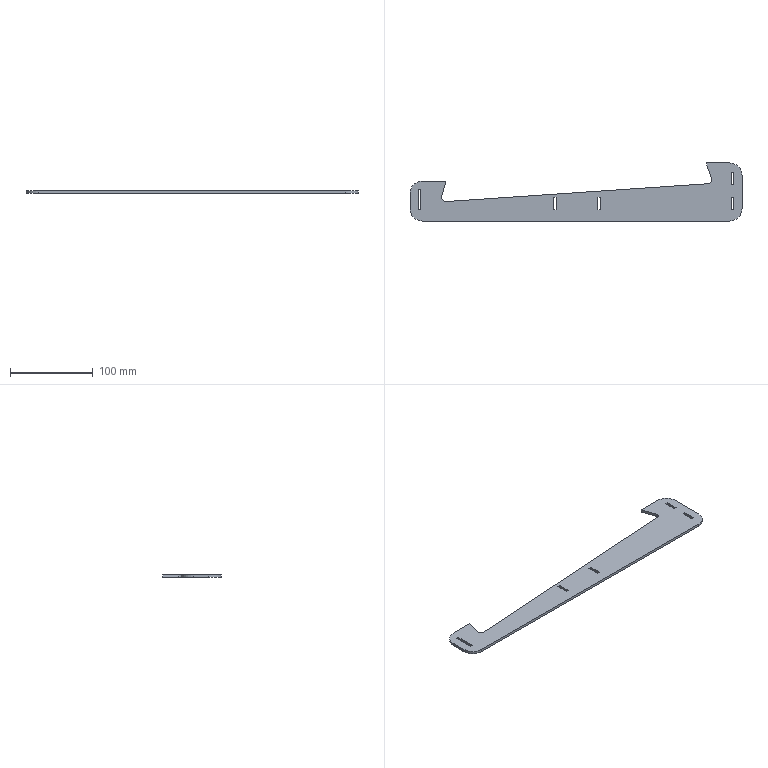Part | SolidWorks | features FlatPattern 1, SMBaseFlange 1, SheetMetal 1 | 1 solid | 36 faces | box 400 x 70 x 3.2 mm | volume 48547 mm3 | plane 29 | cylinder 4 | spline 3 | commonest cylinder face diameters 30 x4
STEP:
#1=CARTESIAN_POINT('',(187.397,-161.486,3.2));
#2=VERTEX_POINT('',#1);
#3=CARTESIAN_POINT('',(182.437,-167.928,3.2));
#4=VERTEX_POINT('',#3);
#5=CARTESIAN_POINT('',(187.397,-161.486,3.2));
#6=CARTESIAN_POINT('',(187.466,-161.697,3.2));
#7=CARTESIAN_POINT('',(187.548,-161.997,3.2));
#8=CARTESIAN_POINT('',(187.606,-162.322,3.2));
#9=CARTESIAN_POINT('',(187.625,-162.479,3.2));
#10=CARTESIAN_POINT('',(187.633,-162.555,3.2));
#11=CARTESIAN_POINT('',(187.635,-162.588,3.2));
#12=CARTESIAN_POINT('',(187.637,-162.609,3.2));
#13=CARTESIAN_POINT('',(187.638,-162.619,3.2));
#14=CARTESIAN_POINT('',(187.651,-162.822,3.2));
#15=CARTESIAN_POINT('',(187.65,-163.111,3.2));
#16=CARTESIAN_POINT('',(187.614,-163.449,3.2));
#17=CARTESIAN_POINT('',(187.591,-163.594,3.2));
#18=CARTESIAN_POINT('',(187.575,-163.691,3.2));
#19=CARTESIAN_POINT('',(187.565,-163.741,3.2));
#20=CARTESIAN_POINT('',(187.476,-164.167,3.2));
#21=CARTESIAN_POINT('',(187.29,-164.713,3.2));
#22=CARTESIAN_POINT('',(186.955,-165.309,3.2));
#23=CARTESIAN_POINT('',(186.758,-165.597,3.2));
#24=CARTESIAN_POINT('',(186.652,-165.738,3.2));
#25=CARTESIAN_POINT('',(186.605,-165.799,3.2));
#26=CARTESIAN_POINT('',(186.573,-165.838,3.2));
#27=CARTESIAN_POINT('',(186.557,-165.859,3.2));
#28=CARTESIAN_POINT('',(186.294,-166.181,3.2));
#29=CARTESIAN_POINT('',(185.879,-166.59,3.2));
#30=CARTESIAN_POINT('',(185.317,-166.988,3.2));
#31=CARTESIAN_POINT('',(185.06,-167.142,3.2));
#32=CARTESIAN_POINT('',(184.885,-167.24,3.2));
#33=CARTESIAN_POINT('',(184.794,-167.288,3.2));
#34=CARTESIAN_POINT('',(184.524,-167.423,3.2));
#35=CARTESIAN_POINT('',(184.251,-167.54,3.2));
#36=CARTESIAN_POINT('',(183.927,-167.648,3.2));
#37=CARTESIAN_POINT('',(183.764,-167.695,3.2));
#38=CARTESIAN_POINT('',(183.682,-167.717,3.2));
#39=CARTESIAN_POINT('',(183.641,-167.727,3.2));
#40=CARTESIAN_POINT('',(183.623,-167.731,3.2));
#41=CARTESIAN_POINT('',(183.611,-167.734,3.2));
#42=CARTESIAN_POINT('',(183.603,-167.736,3.2));
#43=CARTESIAN_POINT('',(183.346,-167.797,3.2));
#44=CARTESIAN_POINT('',(182.958,-167.861,3.2));
#45=CARTESIAN_POINT('',(182.437,-167.928,3.2));
#46=B_SPLINE_CURVE_WITH_KNOTS('',3,(#5,#6,#7,#8,#9,#10,#11,#12,#13,#14,#15,#16,#17,#18,#19,#20,#21,#22,#23,#24,#25,#26,#27,#28,#29,#30,#31,#32,#33,#34,#35,#36,#37,#38,#39,#40,#41,#42,#43,#44,#45),.UNSPECIFIED.,.F.,.F.,(4,1,1,1,1,2,2,1,1,2,2,1,1,1,1,2,2,1,1,2,2,1,1,1,1,1,2,2,4),(0.,0.0625,0.09375,0.1094,0.1172,0.1211,0.125,0.1875,0.2188,0.2344,0.25,0.375,0.4375,0.4688,0.4844,0.4922,0.5,0.625,0.6875,0.7188,0.75,0.8125,0.8438,0.8594,0.8672,0.8711,0.873,0.875,1.),.UNSPECIFIED.);
#47=EDGE_CURVE('',#2,#4,#46,.T.);
#48=ORIENTED_EDGE('',*,*,#47,.T.);
#49=CARTESIAN_POINT('',(-132.11,-189.357,3.2));
#50=VERTEX_POINT('',#49);
#51=CARTESIAN_POINT('',(182.437,-167.928,3.2));
#52=CARTESIAN_POINT('',(77.588,-175.071,3.2));
#53=CARTESIAN_POINT('',(-27.261,-182.214,3.2));
#54=CARTESIAN_POINT('',(-132.11,-189.357,3.2));
#55=B_SPLINE_CURVE_WITH_KNOTS('',3,(#51,#52,#53,#54),.UNSPECIFIED.,.F.,.F.,(4,4),(0.,1.),.UNSPECIFIED.);
#56=EDGE_CURVE('',#4,#50,#55,.T.);
#57=ORIENTED_EDGE('',*,*,#56,.T.);
#58=CARTESIAN_POINT('',(-137.953,-183.594,3.2));
#59=VERTEX_POINT('',#58);
#60=CARTESIAN_POINT('',(-132.11,-189.357,3.2));
#61=CARTESIAN_POINT('',(-132.532,-189.381,3.2));
#62=CARTESIAN_POINT('',(-133.143,-189.364,3.2));
#63=CARTESIAN_POINT('',(-133.815,-189.25,3.2));
#64=CARTESIAN_POINT('',(-134.141,-189.169,3.2));
#65=CARTESIAN_POINT('',(-134.302,-189.122,3.2));
#66=CARTESIAN_POINT('',(-134.37,-189.101,3.2));
#67=CARTESIAN_POINT('',(-134.416,-189.087,3.2));
#68=CARTESIAN_POINT('',(-134.437,-189.08,3.2));
#69=CARTESIAN_POINT('',(-134.848,-188.944,3.2));
#70=CARTESIAN_POINT('',(-135.394,-188.697,3.2));
#71=CARTESIAN_POINT('',(-135.969,-188.316,3.2));
#72=CARTESIAN_POINT('',(-136.242,-188.101,3.2));
#73=CARTESIAN_POINT('',(-136.355,-188.004,3.2));
#74=CARTESIAN_POINT('',(-136.43,-187.938,3.2));
#75=CARTESIAN_POINT('',(-136.466,-187.906,3.2));
#76=CARTESIAN_POINT('',(-136.809,-187.588,3.2));
#77=CARTESIAN_POINT('',(-137.202,-187.132,3.2));
#78=CARTESIAN_POINT('',(-137.545,-186.546,3.2));
#79=CARTESIAN_POINT('',(-137.688,-186.239,3.2));
#80=CARTESIAN_POINT('',(-137.743,-186.104,3.2));
#81=CARTESIAN_POINT('',(-137.778,-186.014,3.2));
#82=CARTESIAN_POINT('',(-137.795,-185.97,3.2));
#83=CARTESIAN_POINT('',(-137.879,-185.734,3.2));
#84=CARTESIAN_POINT('',(-137.932,-185.544,3.2));
#85=CARTESIAN_POINT('',(-138.012,-185.161,3.2));
#86=CARTESIAN_POINT('',(-138.038,-184.969,3.2));
#87=CARTESIAN_POINT('',(-138.057,-184.675,3.2));
#88=CARTESIAN_POINT('',(-138.061,-184.528,3.2));
#89=CARTESIAN_POINT('',(-138.057,-184.38,3.2));
#90=CARTESIAN_POINT('',(-138.052,-184.281,3.2));
#91=CARTESIAN_POINT('',(-138.05,-184.24,3.2));
#92=CARTESIAN_POINT('',(-138.031,-184.015,3.2));
#93=CARTESIAN_POINT('',(-138.,-183.815,3.2));
#94=CARTESIAN_POINT('',(-137.953,-183.594,3.2));
#95=B_SPLINE_CURVE_WITH_KNOTS('',3,(#60,#61,#62,#63,#64,#65,#66,#67,#68,#69,#70,#71,#72,#73,#74,#75,#76,#77,#78,#79,#80,#81,#82,#83,#84,#85,#86,#87,#88,#89,#90,#91,#92,#93,#94),.UNSPECIFIED.,.F.,.F.,(4,1,1,1,1,2,2,1,1,1,2,2,1,1,1,2,2,2,2,1,2,2,4),(0.,0.125,0.1875,0.2187,0.2344,0.2422,0.25,0.375,0.4375,0.4687,0.4844,0.5,0.625,0.6875,0.7187,0.7344,0.75,0.8125,0.875,0.9062,0.9219,0.9375,1.),.UNSPECIFIED.);
#96=EDGE_CURVE('',#50,#59,#95,.T.);
#97=ORIENTED_EDGE('',*,*,#96,.T.);
#98=CARTESIAN_POINT('',(-132.905,-164.74,3.2));
#99=VERTEX_POINT('',#98);
#100=CARTESIAN_POINT('',(-137.953,-183.594,3.2));
#101=CARTESIAN_POINT('',(-136.27,-177.309,3.2));
#102=CARTESIAN_POINT('',(-134.588,-171.025,3.2));
#103=CARTESIAN_POINT('',(-132.905,-164.74,3.2));
#104=B_SPLINE_CURVE_WITH_KNOTS('',3,(#100,#101,#102,#103),.UNSPECIFIED.,.F.,.F.,(4,4),(0.,1.),.UNSPECIFIED.);
#105=EDGE_CURVE('',#59,#99,#104,.T.);
#106=ORIENTED_EDGE('',*,*,#105,.T.);
#107=CARTESIAN_POINT('',(-161.142,-164.74,3.2));
#108=VERTEX_POINT('',#107);
#109=CARTESIAN_POINT('',(-132.905,-164.74,3.2));
#110=DIRECTION('',(-1.,0.,0.));
#111=VECTOR('',#110,1000.);
#112=LINE('',#109,#111);
#113=EDGE_CURVE('',#99,#108,#112,.T.);
#114=ORIENTED_EDGE('',*,*,#113,.T.);
#115=CARTESIAN_POINT('',(-176.142,-179.74,3.2));
#116=VERTEX_POINT('',#115);
#117=CARTESIAN_POINT('',(-161.142,-179.74,3.2));
#118=DIRECTION('',(0.,0.,1.));
#119=DIRECTION('',(1.,0.,0.));
#120=AXIS2_PLACEMENT_3D('',#117,#118,#119);
#121=CIRCLE('',#120,15.);
#122=EDGE_CURVE('',#108,#116,#121,.T.);
#123=ORIENTED_EDGE('',*,*,#122,.T.);
#124=CARTESIAN_POINT('',(-176.142,-197.865,3.2));
#125=VERTEX_POINT('',#124);
#126=CARTESIAN_POINT('',(-176.142,-179.74,3.2));
#127=DIRECTION('',(0.,-1.,0.));
#128=VECTOR('',#127,1000.);
#129=LINE('',#126,#128);
#130=EDGE_CURVE('',#116,#125,#129,.T.);
#131=ORIENTED_EDGE('',*,*,#130,.T.);
#132=CARTESIAN_POINT('',(-161.142,-212.865,3.2));
#133=VERTEX_POINT('',#132);
#134=CARTESIAN_POINT('',(-161.142,-197.865,3.2));
#135=DIRECTION('',(0.,0.,1.));
#136=DIRECTION('',(1.,0.,0.));
#137=AXIS2_PLACEMENT_3D('',#134,#135,#136);
#138=CIRCLE('',#137,15.);
#139=EDGE_CURVE('',#125,#133,#138,.T.);
#140=ORIENTED_EDGE('',*,*,#139,.T.);
#141=CARTESIAN_POINT('',(208.858,-212.865,3.2));
#142=VERTEX_POINT('',#141);
#143=CARTESIAN_POINT('',(-161.142,-212.865,3.2));
#144=DIRECTION('',(1.,0.,0.));
#145=VECTOR('',#144,1000.);
#146=LINE('',#143,#145);
#147=EDGE_CURVE('',#133,#142,#146,.T.);
#148=ORIENTED_EDGE('',*,*,#147,.T.);
#149=CARTESIAN_POINT('',(223.858,-197.865,3.2));
#150=VERTEX_POINT('',#149);
#151=CARTESIAN_POINT('',(208.858,-197.865,3.2));
#152=DIRECTION('',(0.,0.,1.));
#153=DIRECTION('',(1.,0.,0.));
#154=AXIS2_PLACEMENT_3D('',#151,#152,#153);
#155=CIRCLE('',#154,15.);
#156=EDGE_CURVE('',#142,#150,#155,.T.);
#157=ORIENTED_EDGE('',*,*,#156,.T.);
#158=CARTESIAN_POINT('',(223.858,-157.865,3.2));
#159=VERTEX_POINT('',#158);
#160=CARTESIAN_POINT('',(223.858,-197.865,3.2));
#161=DIRECTION('',(0.,1.,0.));
#162=VECTOR('',#161,1000.);
#163=LINE('',#160,#162);
#164=EDGE_CURVE('',#150,#159,#163,.T.);
#165=ORIENTED_EDGE('',*,*,#164,.T.);
#166=CARTESIAN_POINT('',(208.858,-142.865,3.2));
#167=VERTEX_POINT('',#166);
#168=CARTESIAN_POINT('',(208.858,-157.865,3.2));
#169=DIRECTION('',(0.,0.,1.));
#170=DIRECTION('',(1.,0.,0.));
#171=AXIS2_PLACEMENT_3D('',#168,#169,#170);
#172=CIRCLE('',#171,15.);
#173=EDGE_CURVE('',#159,#167,#172,.T.);
#174=ORIENTED_EDGE('',*,*,#173,.T.);
#175=CARTESIAN_POINT('',(180.62,-142.865,3.2));
#176=VERTEX_POINT('',#175);
#177=CARTESIAN_POINT('',(208.858,-142.865,3.2));
#178=DIRECTION('',(-1.,0.,0.));
#179=VECTOR('',#178,1000.);
#180=LINE('',#177,#179);
#181=EDGE_CURVE('',#167,#176,#180,.T.);
#182=ORIENTED_EDGE('',*,*,#181,.T.);
#183=CARTESIAN_POINT('',(180.62,-142.865,3.2));
#184=CARTESIAN_POINT('',(184.003,-152.159,3.2));
#185=CARTESIAN_POINT('',(187.397,-161.486,3.2));
#186=B_SPLINE_CURVE_WITH_KNOTS('',2,(#183,#184,#185),.UNSPECIFIED.,.F.,.F.,(3,3),(0.5261,0.5262),.UNSPECIFIED.);
#187=EDGE_CURVE('',#176,#2,#186,.T.);
#188=ORIENTED_EDGE('',*,*,#187,.T.);
#189=EDGE_LOOP('',(#48,#57,#97,#106,#114,#123,#131,#140,#148,#157,#165,#174,#182,#188));
#190=FACE_OUTER_BOUND('',#189,.T.);
#191=CARTESIAN_POINT('',(-166.142,-199.357,3.2));
#192=VERTEX_POINT('',#191);
#193=CARTESIAN_POINT('',(-162.942,-199.357,3.2));
#194=VERTEX_POINT('',#193);
#195=CARTESIAN_POINT('',(-166.142,-199.357,3.2));
#196=DIRECTION('',(1.,0.,0.));
#197=VECTOR('',#196,1000.);
#198=LINE('',#195,#197);
#199=EDGE_CURVE('',#192,#194,#198,.T.);
#200=ORIENTED_EDGE('',*,*,#199,.F.);
#201=CARTESIAN_POINT('',(-166.142,-174.357,3.2));
#202=VERTEX_POINT('',#201);
#203=CARTESIAN_POINT('',(-166.142,-174.357,3.2));
#204=DIRECTION('',(0.,-1.,0.));
#205=VECTOR('',#204,1000.);
#206=LINE('',#203,#205);
#207=EDGE_CURVE('',#202,#192,#206,.T.);
#208=ORIENTED_EDGE('',*,*,#207,.F.);
#209=CARTESIAN_POINT('',(-162.942,-174.357,3.2));
#210=VERTEX_POINT('',#209);
#211=CARTESIAN_POINT('',(-166.142,-174.357,3.2));
#212=DIRECTION('',(-1.,0.,0.));
#213=VECTOR('',#212,1000.);
#214=LINE('',#211,#213);
#215=EDGE_CURVE('',#210,#202,#214,.T.);
#216=ORIENTED_EDGE('',*,*,#215,.F.);
#217=CARTESIAN_POINT('',(-162.942,-174.357,3.2));
#218=DIRECTION('',(0.,1.,0.));
#219=VECTOR('',#218,1000.);
#220=LINE('',#217,#219);
#221=EDGE_CURVE('',#194,#210,#220,.T.);
#222=ORIENTED_EDGE('',*,*,#221,.F.);
#223=EDGE_LOOP('',(#200,#208,#216,#222));
#224=FACE_BOUND('',#223,.T.);
#225=CARTESIAN_POINT('',(-3.2,-199.357,3.2));
#226=VERTEX_POINT('',#225);
#227=CARTESIAN_POINT('',(0.,-199.357,3.2));
#228=VERTEX_POINT('',#227);
#229=CARTESIAN_POINT('',(-3.2,-199.357,3.2));
#230=DIRECTION('',(1.,0.,0.));
#231=VECTOR('',#230,1000.);
#232=LINE('',#229,#231);
#233=EDGE_CURVE('',#226,#228,#232,.T.);
#234=ORIENTED_EDGE('',*,*,#233,.F.);
#235=CARTESIAN_POINT('',(-3.2,-184.357,3.2));
#236=VERTEX_POINT('',#235);
#237=CARTESIAN_POINT('',(-3.2,-184.357,3.2));
#238=DIRECTION('',(0.,-1.,0.));
#239=VECTOR('',#238,1000.);
#240=LINE('',#237,#239);
#241=EDGE_CURVE('',#236,#226,#240,.T.);
#242=ORIENTED_EDGE('',*,*,#241,.F.);
#243=CARTESIAN_POINT('',(0.,-184.357,3.2));
#244=VERTEX_POINT('',#243);
#245=CARTESIAN_POINT('',(-3.2,-184.357,3.2));
#246=DIRECTION('',(-1.,0.,0.));
#247=VECTOR('',#246,1000.);
#248=LINE('',#245,#247);
#249=EDGE_CURVE('',#244,#236,#248,.T.);
#250=ORIENTED_EDGE('',*,*,#249,.F.);
#251=CARTESIAN_POINT('',(0.,-184.357,3.2));
#252=DIRECTION('',(0.,1.,0.));
#253=VECTOR('',#252,1000.);
#254=LINE('',#251,#253);
#255=EDGE_CURVE('',#228,#244,#254,.T.);
#256=ORIENTED_EDGE('',*,*,#255,.F.);
#257=EDGE_LOOP('',(#234,#242,#250,#256));
#258=FACE_BOUND('',#257,.T.);
#259=CARTESIAN_POINT('',(50.,-199.357,3.2));
#260=VERTEX_POINT('',#259);
#261=CARTESIAN_POINT('',(53.2,-199.357,3.2));
#262=VERTEX_POINT('',#261);
#263=CARTESIAN_POINT('',(50.,-199.357,3.2));
#264=DIRECTION('',(1.,0.,0.));
#265=VECTOR('',#264,1000.);
#266=LINE('',#263,#265);
#267=EDGE_CURVE('',#260,#262,#266,.T.);
#268=ORIENTED_EDGE('',*,*,#267,.F.);
#269=CARTESIAN_POINT('',(50.,-184.357,3.2));
#270=VERTEX_POINT('',#269);
#271=CARTESIAN_POINT('',(50.,-184.357,3.2));
#272=DIRECTION('',(0.,-1.,0.));
#273=VECTOR('',#272,1000.);
#274=LINE('',#271,#273);
#275=EDGE_CURVE('',#270,#260,#274,.T.);
#276=ORIENTED_EDGE('',*,*,#275,.F.);
#277=CARTESIAN_POINT('',(53.2,-184.357,3.2));
#278=VERTEX_POINT('',#277);
#279=CARTESIAN_POINT('',(50.,-184.357,3.2));
#280=DIRECTION('',(-1.,0.,0.));
#281=VECTOR('',#280,1000.);
#282=LINE('',#279,#281);
#283=EDGE_CURVE('',#278,#270,#282,.T.);
#284=ORIENTED_EDGE('',*,*,#283,.F.);
#285=CARTESIAN_POINT('',(53.2,-184.357,3.2));
#286=DIRECTION('',(0.,1.,0.));
#287=VECTOR('',#286,1000.);
#288=LINE('',#285,#287);
#289=EDGE_CURVE('',#262,#278,#288,.T.);
#290=ORIENTED_EDGE('',*,*,#289,.F.);
#291=EDGE_LOOP('',(#268,#276,#284,#290));
#292=FACE_BOUND('',#291,.T.);
#293=CARTESIAN_POINT('',(210.658,-169.357,3.2));
#294=VERTEX_POINT('',#293);
#295=CARTESIAN_POINT('',(213.858,-169.357,3.2));
#296=VERTEX_POINT('',#295);
#297=CARTESIAN_POINT('',(210.658,-169.357,3.2));
#298=DIRECTION('',(1.,0.,0.));
#299=VECTOR('',#298,1000.);
#300=LINE('',#297,#299);
#301=EDGE_CURVE('',#294,#296,#300,.T.);
#302=ORIENTED_EDGE('',*,*,#301,.F.);
#303=CARTESIAN_POINT('',(210.658,-154.357,3.2));
#304=VERTEX_POINT('',#303);
#305=CARTESIAN_POINT('',(210.658,-154.357,3.2));
#306=DIRECTION('',(0.,-1.,0.));
#307=VECTOR('',#306,1000.);
#308=LINE('',#305,#307);
#309=EDGE_CURVE('',#304,#294,#308,.T.);
#310=ORIENTED_EDGE('',*,*,#309,.F.);
#311=CARTESIAN_POINT('',(213.858,-154.357,3.2));
#312=VERTEX_POINT('',#311);
#313=CARTESIAN_POINT('',(210.658,-154.357,3.2));
#314=DIRECTION('',(-1.,0.,0.));
#315=VECTOR('',#314,1000.);
#316=LINE('',#313,#315);
#317=EDGE_CURVE('',#312,#304,#316,.T.);
#318=ORIENTED_EDGE('',*,*,#317,.F.);
#319=CARTESIAN_POINT('',(213.858,-154.357,3.2));
#320=DIRECTION('',(0.,1.,0.));
#321=VECTOR('',#320,1000.);
#322=LINE('',#319,#321);
#323=EDGE_CURVE('',#296,#312,#322,.T.);
#324=ORIENTED_EDGE('',*,*,#323,.F.);
#325=EDGE_LOOP('',(#302,#310,#318,#324));
#326=FACE_BOUND('',#325,.T.);
#327=CARTESIAN_POINT('',(210.658,-199.357,3.2));
#328=VERTEX_POINT('',#327);
#329=CARTESIAN_POINT('',(213.858,-199.357,3.2));
#330=VERTEX_POINT('',#329);
#331=CARTESIAN_POINT('',(210.658,-199.357,3.2));
#332=DIRECTION('',(1.,0.,0.));
#333=VECTOR('',#332,1000.);
#334=LINE('',#331,#333);
#335=EDGE_CURVE('',#328,#330,#334,.T.);
#336=ORIENTED_EDGE('',*,*,#335,.F.);
#337=CARTESIAN_POINT('',(210.658,-184.357,3.2));
#338=VERTEX_POINT('',#337);
#339=CARTESIAN_POINT('',(210.658,-184.357,3.2));
#340=DIRECTION('',(0.,-1.,0.));
#341=VECTOR('',#340,1000.);
#342=LINE('',#339,#341);
#343=EDGE_CURVE('',#338,#328,#342,.T.);
#344=ORIENTED_EDGE('',*,*,#343,.F.);
#345=CARTESIAN_POINT('',(213.858,-184.357,3.2));
#346=VERTEX_POINT('',#345);
#347=CARTESIAN_POINT('',(210.658,-184.357,3.2));
#348=DIRECTION('',(-1.,0.,0.));
#349=VECTOR('',#348,1000.);
#350=LINE('',#347,#349);
#351=EDGE_CURVE('',#346,#338,#350,.T.);
#352=ORIENTED_EDGE('',*,*,#351,.F.);
#353=CARTESIAN_POINT('',(213.858,-184.357,3.2));
#354=DIRECTION('',(0.,1.,0.));
#355=VECTOR('',#354,1000.);
#356=LINE('',#353,#355);
#357=EDGE_CURVE('',#330,#346,#356,.T.);
#358=ORIENTED_EDGE('',*,*,#357,.F.);
#359=EDGE_LOOP('',(#336,#344,#352,#358));
#360=FACE_BOUND('',#359,.T.);
#361=CARTESIAN_POINT('',(186.541,-165.878,3.2));
#362=DIRECTION('',(0.,0.,1.));
#363=DIRECTION('',(1.,0.,0.));
#364=AXIS2_PLACEMENT_3D('',#361,#362,#363);
#365=PLANE('',#364);
#366=ADVANCED_FACE('',(#190,#224,#258,#292,#326,#360),#365,.T.);
#367=CARTESIAN_POINT('',(210.658,-154.357,0.));
#368=VERTEX_POINT('',#367);
#369=CARTESIAN_POINT('',(210.658,-169.357,0.));
#370=VERTEX_POINT('',#369);
#371=CARTESIAN_POINT('',(210.658,-154.357,0.));
#372=DIRECTION('',(0.,-1.,0.));
#373=VECTOR('',#372,1000.);
#374=LINE('',#371,#373);
#375=EDGE_CURVE('',#368,#370,#374,.T.);
#376=ORIENTED_EDGE('',*,*,#375,.T.);
#377=CARTESIAN_POINT('',(213.858,-169.357,0.));
#378=VERTEX_POINT('',#377);
#379=CARTESIAN_POINT('',(210.658,-169.357,0.));
#380=DIRECTION('',(1.,0.,0.));
#381=VECTOR('',#380,1000.);
#382=LINE('',#379,#381);
#383=EDGE_CURVE('',#370,#378,#382,.T.);
#384=ORIENTED_EDGE('',*,*,#383,.T.);
#385=CARTESIAN_POINT('',(213.858,-154.357,0.));
#386=VERTEX_POINT('',#385);
#387=CARTESIAN_POINT('',(213.858,-154.357,0.));
#388=DIRECTION('',(0.,1.,0.));
#389=VECTOR('',#388,1000.);
#390=LINE('',#387,#389);
#391=EDGE_CURVE('',#378,#386,#390,.T.);
#392=ORIENTED_EDGE('',*,*,#391,.T.);
#393=CARTESIAN_POINT('',(210.658,-154.357,0.));
#394=DIRECTION('',(-1.,0.,0.));
#395=VECTOR('',#394,1000.);
#396=LINE('',#393,#395);
#397=EDGE_CURVE('',#386,#368,#396,.T.);
#398=ORIENTED_EDGE('',*,*,#397,.T.);
#399=EDGE_LOOP('',(#376,#384,#392,#398));
#400=FACE_BOUND('',#399,.T.);
#401=CARTESIAN_POINT('',(-3.2,-184.357,0.));
#402=VERTEX_POINT('',#401);
#403=CARTESIAN_POINT('',(-3.2,-199.357,0.));
#404=VERTEX_POINT('',#403);
#405=CARTESIAN_POINT('',(-3.2,-184.357,0.));
#406=DIRECTION('',(0.,-1.,0.));
#407=VECTOR('',#406,1000.);
#408=LINE('',#405,#407);
#409=EDGE_CURVE('',#402,#404,#408,.T.);
#410=ORIENTED_EDGE('',*,*,#409,.T.);
#411=CARTESIAN_POINT('',(0.,-199.357,0.));
#412=VERTEX_POINT('',#411);
#413=CARTESIAN_POINT('',(-3.2,-199.357,0.));
#414=DIRECTION('',(1.,0.,0.));
#415=VECTOR('',#414,1000.);
#416=LINE('',#413,#415);
#417=EDGE_CURVE('',#404,#412,#416,.T.);
#418=ORIENTED_EDGE('',*,*,#417,.T.);
#419=CARTESIAN_POINT('',(0.,-184.357,0.));
#420=VERTEX_POINT('',#419);
#421=CARTESIAN_POINT('',(0.,-184.357,0.));
#422=DIRECTION('',(0.,1.,0.));
#423=VECTOR('',#422,1000.);
#424=LINE('',#421,#423);
#425=EDGE_CURVE('',#412,#420,#424,.T.);
#426=ORIENTED_EDGE('',*,*,#425,.T.);
#427=CARTESIAN_POINT('',(-3.2,-184.357,0.));
#428=DIRECTION('',(-1.,0.,0.));
#429=VECTOR('',#428,1000.);
#430=LINE('',#427,#429);
#431=EDGE_CURVE('',#420,#402,#430,.T.);
#432=ORIENTED_EDGE('',*,*,#431,.T.);
#433=EDGE_LOOP('',(#410,#418,#426,#432));
#434=FACE_BOUND('',#433,.T.);
#435=CARTESIAN_POINT('',(187.397,-161.486,0.));
#436=VERTEX_POINT('',#435);
#437=CARTESIAN_POINT('',(182.437,-167.928,0.));
#438=VERTEX_POINT('',#437);
#439=CARTESIAN_POINT('',(187.397,-161.486,0.));
#440=CARTESIAN_POINT('',(187.445,-161.632,0.));
#441=CARTESIAN_POINT('',(187.544,-161.932,0.));
#442=CARTESIAN_POINT('',(187.628,-162.413,0.));
#443=CARTESIAN_POINT('',(187.659,-162.932,0.));
#444=CARTESIAN_POINT('',(187.61,-163.626,0.));
#445=CARTESIAN_POINT('',(187.39,-164.497,0.));
#446=CARTESIAN_POINT('',(186.881,-165.491,0.));
#447=CARTESIAN_POINT('',(186.11,-166.411,0.));
#448=CARTESIAN_POINT('',(185.064,-167.197,0.));
#449=CARTESIAN_POINT('',(183.813,-167.752,0.));
#450=CARTESIAN_POINT('',(182.885,-167.87,0.));
#451=CARTESIAN_POINT('',(182.437,-167.928,0.));
#452=B_SPLINE_CURVE_WITH_KNOTS('',3,(#439,#440,#441,#442,#443,#444,#445,#446,#447,#448,#449,#450,#451),.UNSPECIFIED.,.F.,.F.,(4,1,1,1,1,1,1,1,1,1,4),(0.,0.04871,0.1004,0.1558,0.2156,0.3245,0.4429,0.5702,0.7032,0.8565,1.),.UNSPECIFIED.);
#453=EDGE_CURVE('',#436,#438,#452,.T.);
#454=ORIENTED_EDGE('',*,*,#453,.F.);
#455=CARTESIAN_POINT('',(180.62,-142.865,0.));
#456=VERTEX_POINT('',#455);
#457=CARTESIAN_POINT('',(180.62,-142.865,0.));
#458=CARTESIAN_POINT('',(184.003,-152.159,0.));
#459=CARTESIAN_POINT('',(187.397,-161.486,0.));
#460=B_SPLINE_CURVE_WITH_KNOTS('',2,(#457,#458,#459),.UNSPECIFIED.,.F.,.F.,(3,3),(0.5261,0.5262),.UNSPECIFIED.);
#461=EDGE_CURVE('',#456,#436,#460,.T.);
#462=ORIENTED_EDGE('',*,*,#461,.F.);
#463=CARTESIAN_POINT('',(208.858,-142.865,0.));
#464=VERTEX_POINT('',#463);
#465=CARTESIAN_POINT('',(208.858,-142.865,0.));
#466=DIRECTION('',(-1.,0.,0.));
#467=VECTOR('',#466,1000.);
#468=LINE('',#465,#467);
#469=EDGE_CURVE('',#464,#456,#468,.T.);
#470=ORIENTED_EDGE('',*,*,#469,.F.);
#471=CARTESIAN_POINT('',(223.858,-157.865,0.));
#472=VERTEX_POINT('',#471);
#473=CARTESIAN_POINT('',(208.858,-157.865,0.));
#474=DIRECTION('',(0.,0.,1.));
#475=DIRECTION('',(1.,0.,0.));
#476=AXIS2_PLACEMENT_3D('',#473,#474,#475);
#477=CIRCLE('',#476,15.);
#478=EDGE_CURVE('',#472,#464,#477,.T.);
#479=ORIENTED_EDGE('',*,*,#478,.F.);
#480=CARTESIAN_POINT('',(223.858,-197.865,0.));
#481=VERTEX_POINT('',#480);
#482=CARTESIAN_POINT('',(223.858,-197.865,0.));
#483=DIRECTION('',(0.,1.,0.));
#484=VECTOR('',#483,1000.);
#485=LINE('',#482,#484);
#486=EDGE_CURVE('',#481,#472,#485,.T.);
#487=ORIENTED_EDGE('',*,*,#486,.F.);
#488=CARTESIAN_POINT('',(208.858,-212.865,0.));
#489=VERTEX_POINT('',#488);
#490=CARTESIAN_POINT('',(208.858,-197.865,0.));
#491=DIRECTION('',(0.,0.,1.));
#492=DIRECTION('',(1.,0.,0.));
#493=AXIS2_PLACEMENT_3D('',#490,#491,#492);
#494=CIRCLE('',#493,15.);
#495=EDGE_CURVE('',#489,#481,#494,.T.);
#496=ORIENTED_EDGE('',*,*,#495,.F.);
#497=CARTESIAN_POINT('',(-161.142,-212.865,0.));
#498=VERTEX_POINT('',#497);
#499=CARTESIAN_POINT('',(-161.142,-212.865,0.));
#500=DIRECTION('',(1.,0.,0.));
#501=VECTOR('',#500,1000.);
#502=LINE('',#499,#501);
#503=EDGE_CURVE('',#498,#489,#502,.T.);
#504=ORIENTED_EDGE('',*,*,#503,.F.);
#505=CARTESIAN_POINT('',(-176.142,-197.865,0.));
#506=VERTEX_POINT('',#505);
#507=CARTESIAN_POINT('',(-161.142,-197.865,0.));
#508=DIRECTION('',(0.,0.,1.));
#509=DIRECTION('',(1.,0.,0.));
#510=AXIS2_PLACEMENT_3D('',#507,#508,#509);
#511=CIRCLE('',#510,15.);
#512=EDGE_CURVE('',#506,#498,#511,.T.);
#513=ORIENTED_EDGE('',*,*,#512,.F.);
#514=CARTESIAN_POINT('',(-176.142,-179.74,0.));
#515=VERTEX_POINT('',#514);
#516=CARTESIAN_POINT('',(-176.142,-179.74,0.));
#517=DIRECTION('',(0.,-1.,0.));
#518=VECTOR('',#517,1000.);
#519=LINE('',#516,#518);
#520=EDGE_CURVE('',#515,#506,#519,.T.);
#521=ORIENTED_EDGE('',*,*,#520,.F.);
#522=CARTESIAN_POINT('',(-161.142,-164.74,0.));
#523=VERTEX_POINT('',#522);
#524=CARTESIAN_POINT('',(-161.142,-179.74,0.));
#525=DIRECTION('',(0.,0.,1.));
#526=DIRECTION('',(1.,0.,0.));
#527=AXIS2_PLACEMENT_3D('',#524,#525,#526);
#528=CIRCLE('',#527,15.);
#529=EDGE_CURVE('',#523,#515,#528,.T.);
#530=ORIENTED_EDGE('',*,*,#529,.F.);
#531=CARTESIAN_POINT('',(-132.905,-164.74,0.));
#532=VERTEX_POINT('',#531);
#533=CARTESIAN_POINT('',(-132.905,-164.74,0.));
#534=DIRECTION('',(-1.,0.,0.));
#535=VECTOR('',#534,1000.);
#536=LINE('',#533,#535);
#537=EDGE_CURVE('',#532,#523,#536,.T.);
#538=ORIENTED_EDGE('',*,*,#537,.F.);
#539=CARTESIAN_POINT('',(-137.953,-183.594,0.));
#540=VERTEX_POINT('',#539);
#541=CARTESIAN_POINT('',(-137.953,-183.594,0.));
#542=CARTESIAN_POINT('',(-136.27,-177.309,0.));
#543=CARTESIAN_POINT('',(-134.588,-171.025,0.));
#544=CARTESIAN_POINT('',(-132.905,-164.74,0.));
#545=B_SPLINE_CURVE_WITH_KNOTS('',3,(#541,#542,#543,#544),.UNSPECIFIED.,.F.,.F.,(4,4),(0.,1.),.UNSPECIFIED.);
#546=EDGE_CURVE('',#540,#532,#545,.T.);
#547=ORIENTED_EDGE('',*,*,#546,.F.);
#548=CARTESIAN_POINT('',(-132.11,-189.357,0.));
#549=VERTEX_POINT('',#548);
#550=CARTESIAN_POINT('',(-132.11,-189.357,0.));
#551=CARTESIAN_POINT('',(-132.186,-189.361,0.));
#552=CARTESIAN_POINT('',(-132.337,-189.37,0.));
#553=CARTESIAN_POINT('',(-132.567,-189.373,0.));
#554=CARTESIAN_POINT('',(-132.8,-189.369,0.));
#555=CARTESIAN_POINT('',(-133.037,-189.356,0.));
#556=CARTESIAN_POINT('',(-133.275,-189.333,0.));
#557=CARTESIAN_POINT('',(-133.654,-189.282,0.));
#558=CARTESIAN_POINT('',(-134.174,-189.172,0.));
#559=CARTESIAN_POINT('',(-135.008,-188.891,0.));
#560=CARTESIAN_POINT('',(-135.956,-188.375,0.));
#561=CARTESIAN_POINT('',(-136.744,-187.674,0.));
#562=CARTESIAN_POINT('',(-137.242,-187.044,0.));
#563=CARTESIAN_POINT('',(-137.548,-186.546,0.));
#564=CARTESIAN_POINT('',(-137.782,-186.036,0.));
#565=CARTESIAN_POINT('',(-137.947,-185.512,0.));
#566=CARTESIAN_POINT('',(-138.041,-184.996,0.));
#567=CARTESIAN_POINT('',(-138.066,-184.548,0.));
#568=CARTESIAN_POINT('',(-138.049,-184.178,0.));
#569=CARTESIAN_POINT('',(-138.013,-183.88,0.));
#570=CARTESIAN_POINT('',(-137.973,-183.688,0.));
#571=CARTESIAN_POINT('',(-137.953,-183.594,0.));
#572=B_SPLINE_CURVE_WITH_KNOTS('',3,(#550,#551,#552,#553,#554,#555,#556,#557,#558,#559,#560,#561,#562,#563,#564,#565,#566,#567,#568,#569,#570,#571),.UNSPECIFIED.,.F.,.F.,(4,1,1,1,1,1,1,1,1,1,1,1,1,1,1,1,1,1,1,4),(0.,0.02376,0.04786,0.07231,0.09712,0.1223,0.1479,0.2174,0.2893,0.4245,0.5536,0.618,0.6781,0.7387,0.7962,0.8526,0.9055,0.9385,0.9699,1.),.UNSPECIFIED.);
#573=EDGE_CURVE('',#549,#540,#572,.T.);
#574=ORIENTED_EDGE('',*,*,#573,.F.);
#575=CARTESIAN_POINT('',(182.437,-167.928,0.));
#576=CARTESIAN_POINT('',(77.588,-175.071,0.));
#577=CARTESIAN_POINT('',(-27.261,-182.214,0.));
#578=CARTESIAN_POINT('',(-132.11,-189.357,0.));
#579=B_SPLINE_CURVE_WITH_KNOTS('',3,(#575,#576,#577,#578),.UNSPECIFIED.,.F.,.F.,(4,4),(0.,1.),.UNSPECIFIED.);
#580=EDGE_CURVE('',#438,#549,#579,.T.);
#581=ORIENTED_EDGE('',*,*,#580,.F.);
#582=EDGE_LOOP('',(#454,#462,#470,#479,#487,#496,#504,#513,#521,#530,#538,#547,#574,#581));
#583=FACE_OUTER_BOUND('',#582,.T.);
#584=CARTESIAN_POINT('',(-166.142,-174.357,0.));
#585=VERTEX_POINT('',#584);
#586=CARTESIAN_POINT('',(-166.142,-199.357,0.));
#587=VERTEX_POINT('',#586);
#588=CARTESIAN_POINT('',(-166.142,-174.357,0.));
#589=DIRECTION('',(0.,-1.,0.));
#590=VECTOR('',#589,1000.);
#591=LINE('',#588,#590);
#592=EDGE_CURVE('',#585,#587,#591,.T.);
#593=ORIENTED_EDGE('',*,*,#592,.T.);
#594=CARTESIAN_POINT('',(-162.942,-199.357,0.));
#595=VERTEX_POINT('',#594);
#596=CARTESIAN_POINT('',(-166.142,-199.357,0.));
#597=DIRECTION('',(1.,0.,0.));
#598=VECTOR('',#597,1000.);
#599=LINE('',#596,#598);
#600=EDGE_CURVE('',#587,#595,#599,.T.);
#601=ORIENTED_EDGE('',*,*,#600,.T.);
#602=CARTESIAN_POINT('',(-162.942,-174.357,0.));
#603=VERTEX_POINT('',#602);
#604=CARTESIAN_POINT('',(-162.942,-174.357,0.));
#605=DIRECTION('',(0.,1.,0.));
#606=VECTOR('',#605,1000.);
#607=LINE('',#604,#606);
#608=EDGE_CURVE('',#595,#603,#607,.T.);
#609=ORIENTED_EDGE('',*,*,#608,.T.);
#610=CARTESIAN_POINT('',(-166.142,-174.357,0.));
#611=DIRECTION('',(-1.,0.,0.));
#612=VECTOR('',#611,1000.);
#613=LINE('',#610,#612);
#614=EDGE_CURVE('',#603,#585,#613,.T.);
#615=ORIENTED_EDGE('',*,*,#614,.T.);
#616=EDGE_LOOP('',(#593,#601,#609,#615));
#617=FACE_BOUND('',#616,.T.);
#618=CARTESIAN_POINT('',(50.,-184.357,0.));
#619=VERTEX_POINT('',#618);
#620=CARTESIAN_POINT('',(50.,-199.357,0.));
#621=VERTEX_POINT('',#620);
#622=CARTESIAN_POINT('',(50.,-184.357,0.));
#623=DIRECTION('',(0.,-1.,0.));
#624=VECTOR('',#623,1000.);
#625=LINE('',#622,#624);
#626=EDGE_CURVE('',#619,#621,#625,.T.);
#627=ORIENTED_EDGE('',*,*,#626,.T.);
#628=CARTESIAN_POINT('',(53.2,-199.357,0.));
#629=VERTEX_POINT('',#628);
#630=CARTESIAN_POINT('',(50.,-199.357,0.));
#631=DIRECTION('',(1.,0.,0.));
#632=VECTOR('',#631,1000.);
#633=LINE('',#630,#632);
#634=EDGE_CURVE('',#621,#629,#633,.T.);
#635=ORIENTED_EDGE('',*,*,#634,.T.);
#636=CARTESIAN_POINT('',(53.2,-184.357,0.));
#637=VERTEX_POINT('',#636);
#638=CARTESIAN_POINT('',(53.2,-184.357,0.));
#639=DIRECTION('',(0.,1.,0.));
#640=VECTOR('',#639,1000.);
#641=LINE('',#638,#640);
#642=EDGE_CURVE('',#629,#637,#641,.T.);
#643=ORIENTED_EDGE('',*,*,#642,.T.);
#644=CARTESIAN_POINT('',(50.,-184.357,0.));
#645=DIRECTION('',(-1.,0.,0.));
#646=VECTOR('',#645,1000.);
#647=LINE('',#644,#646);
#648=EDGE_CURVE('',#637,#619,#647,.T.);
#649=ORIENTED_EDGE('',*,*,#648,.T.);
#650=EDGE_LOOP('',(#627,#635,#643,#649));
#651=FACE_BOUND('',#650,.T.);
#652=CARTESIAN_POINT('',(210.658,-184.357,0.));
#653=VERTEX_POINT('',#652);
#654=CARTESIAN_POINT('',(210.658,-199.357,0.));
#655=VERTEX_POINT('',#654);
#656=CARTESIAN_POINT('',(210.658,-184.357,0.));
#657=DIRECTION('',(0.,-1.,0.));
#658=VECTOR('',#657,1000.);
#659=LINE('',#656,#658);
#660=EDGE_CURVE('',#653,#655,#659,.T.);
#661=ORIENTED_EDGE('',*,*,#660,.T.);
#662=CARTESIAN_POINT('',(213.858,-199.357,0.));
#663=VERTEX_POINT('',#662);
#664=CARTESIAN_POINT('',(210.658,-199.357,0.));
#665=DIRECTION('',(1.,0.,0.));
#666=VECTOR('',#665,1000.);
#667=LINE('',#664,#666);
#668=EDGE_CURVE('',#655,#663,#667,.T.);
#669=ORIENTED_EDGE('',*,*,#668,.T.);
#670=CARTESIAN_POINT('',(213.858,-184.357,0.));
#671=VERTEX_POINT('',#670);
#672=CARTESIAN_POINT('',(213.858,-184.357,0.));
#673=DIRECTION('',(0.,1.,0.));
#674=VECTOR('',#673,1000.);
#675=LINE('',#672,#674);
#676=EDGE_CURVE('',#663,#671,#675,.T.);
#677=ORIENTED_EDGE('',*,*,#676,.T.);
#678=CARTESIAN_POINT('',(210.658,-184.357,0.));
#679=DIRECTION('',(-1.,0.,0.));
#680=VECTOR('',#679,1000.);
#681=LINE('',#678,#680);
#682=EDGE_CURVE('',#671,#653,#681,.T.);
#683=ORIENTED_EDGE('',*,*,#682,.T.);
#684=EDGE_LOOP('',(#661,#669,#677,#683));
#685=FACE_BOUND('',#684,.T.);
#686=CARTESIAN_POINT('',(186.541,-165.878,0.));
#687=DIRECTION('',(0.,0.,1.));
#688=DIRECTION('',(1.,0.,0.));
#689=AXIS2_PLACEMENT_3D('',#686,#687,#688);
#690=PLANE('',#689);
#691=ADVANCED_FACE('',(#400,#434,#583,#617,#651,#685),#690,.F.);
#692=ORIENTED_EDGE('',*,*,#453,.T.);
#693=CARTESIAN_POINT('',(182.437,-167.928,3.2));
#694=DIRECTION('',(0.,0.,-1.));
#695=VECTOR('',#694,1000.);
#696=LINE('',#693,#695);
#697=EDGE_CURVE('',#4,#438,#696,.T.);
#698=ORIENTED_EDGE('',*,*,#697,.F.);
#699=ORIENTED_EDGE('',*,*,#47,.F.);
#700=CARTESIAN_POINT('',(187.397,-161.486,3.2));
#701=DIRECTION('',(0.,0.,-1.));
#702=VECTOR('',#701,1000.);
#703=LINE('',#700,#702);
#704=EDGE_CURVE('',#2,#436,#703,.T.);
#705=ORIENTED_EDGE('',*,*,#704,.T.);
#706=EDGE_LOOP('',(#692,#698,#699,#705));
#707=FACE_OUTER_BOUND('',#706,.T.);
#708=CARTESIAN_POINT('',(187.397,-161.486,3.2));
#709=CARTESIAN_POINT('',(187.397,-161.486,0.));
#710=CARTESIAN_POINT('',(187.445,-161.632,3.2));
#711=CARTESIAN_POINT('',(187.445,-161.632,0.));
#712=CARTESIAN_POINT('',(187.544,-161.932,3.2));
#713=CARTESIAN_POINT('',(187.544,-161.932,0.));
#714=CARTESIAN_POINT('',(187.628,-162.413,3.2));
#715=CARTESIAN_POINT('',(187.628,-162.413,0.));
#716=CARTESIAN_POINT('',(187.659,-162.932,3.2));
#717=CARTESIAN_POINT('',(187.659,-162.932,0.));
#718=CARTESIAN_POINT('',(187.61,-163.626,3.2));
#719=CARTESIAN_POINT('',(187.61,-163.626,0.));
#720=CARTESIAN_POINT('',(187.39,-164.497,3.2));
#721=CARTESIAN_POINT('',(187.39,-164.497,0.));
#722=CARTESIAN_POINT('',(186.881,-165.491,3.2));
#723=CARTESIAN_POINT('',(186.881,-165.491,0.));
#724=CARTESIAN_POINT('',(186.11,-166.411,3.2));
#725=CARTESIAN_POINT('',(186.11,-166.411,0.));
#726=CARTESIAN_POINT('',(185.064,-167.197,3.2));
#727=CARTESIAN_POINT('',(185.064,-167.197,0.));
#728=CARTESIAN_POINT('',(183.813,-167.752,3.2));
#729=CARTESIAN_POINT('',(183.813,-167.752,0.));
#730=CARTESIAN_POINT('',(182.885,-167.87,3.2));
#731=CARTESIAN_POINT('',(182.885,-167.87,0.));
#732=CARTESIAN_POINT('',(182.437,-167.928,3.2));
#733=CARTESIAN_POINT('',(182.437,-167.928,0.));
#734=B_SPLINE_SURFACE_WITH_KNOTS('',3,1,((#708,#709),(#710,#711),(#712,#713),(#714,#715),(#716,#717),(#718,#719),(#720,#721),(#722,#723),(#724,#725),(#726,#727),(#728,#729),(#730,#731),(#732,#733)),.UNSPECIFIED.,.F.,.F.,.F.,(4,1,1,1,1,1,1,1,1,1,4),(2,2),(0.,0.04871,0.1004,0.1558,0.2156,0.3245,0.4429,0.5702,0.7032,0.8565,1.),(0.,1.),.UNSPECIFIED.);
#735=ADVANCED_FACE('',(#707),#734,.F.);
#736=ORIENTED_EDGE('',*,*,#580,.T.);
#737=CARTESIAN_POINT('',(-132.11,-189.357,3.2));
#738=DIRECTION('',(0.,0.,-1.));
#739=VECTOR('',#738,1000.);
#740=LINE('',#737,#739);
#741=EDGE_CURVE('',#50,#549,#740,.T.);
#742=ORIENTED_EDGE('',*,*,#741,.F.);
#743=ORIENTED_EDGE('',*,*,#56,.F.);
#744=ORIENTED_EDGE('',*,*,#697,.T.);
#745=EDGE_LOOP('',(#736,#742,#743,#744));
#746=FACE_OUTER_BOUND('',#745,.T.);
#747=CARTESIAN_POINT('',(182.437,-167.928,3.2));
#748=DIRECTION('',(0.06797,-0.9977,0.));
#749=DIRECTION('',(0.9977,0.06797,0.));
#750=AXIS2_PLACEMENT_3D('',#747,#748,#749);
#751=PLANE('',#750);
#752=ADVANCED_FACE('',(#746),#751,.F.);
#753=ORIENTED_EDGE('',*,*,#573,.T.);
#754=CARTESIAN_POINT('',(-137.953,-183.594,3.2));
#755=DIRECTION('',(0.,0.,-1.));
#756=VECTOR('',#755,1000.);
#757=LINE('',#754,#756);
#758=EDGE_CURVE('',#59,#540,#757,.T.);
#759=ORIENTED_EDGE('',*,*,#758,.F.);
#760=ORIENTED_EDGE('',*,*,#96,.F.);
#761=ORIENTED_EDGE('',*,*,#741,.T.);
#762=EDGE_LOOP('',(#753,#759,#760,#761));
#763=FACE_OUTER_BOUND('',#762,.T.);
#764=CARTESIAN_POINT('',(-132.11,-189.357,3.2));
#765=CARTESIAN_POINT('',(-132.11,-189.357,0.));
#766=CARTESIAN_POINT('',(-132.186,-189.361,3.2));
#767=CARTESIAN_POINT('',(-132.186,-189.361,0.));
#768=CARTESIAN_POINT('',(-132.337,-189.37,3.2));
#769=CARTESIAN_POINT('',(-132.337,-189.37,0.));
#770=CARTESIAN_POINT('',(-132.567,-189.373,3.2));
#771=CARTESIAN_POINT('',(-132.567,-189.373,0.));
#772=CARTESIAN_POINT('',(-132.8,-189.369,3.2));
#773=CARTESIAN_POINT('',(-132.8,-189.369,0.));
#774=CARTESIAN_POINT('',(-133.037,-189.356,3.2));
#775=CARTESIAN_POINT('',(-133.037,-189.356,0.));
#776=CARTESIAN_POINT('',(-133.275,-189.333,3.2));
#777=CARTESIAN_POINT('',(-133.275,-189.333,0.));
#778=CARTESIAN_POINT('',(-133.654,-189.282,3.2));
#779=CARTESIAN_POINT('',(-133.654,-189.282,0.));
#780=CARTESIAN_POINT('',(-134.174,-189.172,3.2));
#781=CARTESIAN_POINT('',(-134.174,-189.172,0.));
#782=CARTESIAN_POINT('',(-135.008,-188.891,3.2));
#783=CARTESIAN_POINT('',(-135.008,-188.891,0.));
#784=CARTESIAN_POINT('',(-135.956,-188.375,3.2));
#785=CARTESIAN_POINT('',(-135.956,-188.375,0.));
#786=CARTESIAN_POINT('',(-136.744,-187.674,3.2));
#787=CARTESIAN_POINT('',(-136.744,-187.674,0.));
#788=CARTESIAN_POINT('',(-137.242,-187.044,3.2));
#789=CARTESIAN_POINT('',(-137.242,-187.044,0.));
#790=CARTESIAN_POINT('',(-137.548,-186.546,3.2));
#791=CARTESIAN_POINT('',(-137.548,-186.546,0.));
#792=CARTESIAN_POINT('',(-137.782,-186.036,3.2));
#793=CARTESIAN_POINT('',(-137.782,-186.036,0.));
#794=CARTESIAN_POINT('',(-137.947,-185.512,3.2));
#795=CARTESIAN_POINT('',(-137.947,-185.512,0.));
#796=CARTESIAN_POINT('',(-138.041,-184.996,3.2));
#797=CARTESIAN_POINT('',(-138.041,-184.996,0.));
#798=CARTESIAN_POINT('',(-138.066,-184.548,3.2));
#799=CARTESIAN_POINT('',(-138.066,-184.548,0.));
#800=CARTESIAN_POINT('',(-138.049,-184.178,3.2));
#801=CARTESIAN_POINT('',(-138.049,-184.178,0.));
#802=CARTESIAN_POINT('',(-138.013,-183.88,3.2));
#803=CARTESIAN_POINT('',(-138.013,-183.88,0.));
#804=CARTESIAN_POINT('',(-137.973,-183.688,3.2));
#805=CARTESIAN_POINT('',(-137.973,-183.688,0.));
#806=CARTESIAN_POINT('',(-137.953,-183.594,3.2));
#807=CARTESIAN_POINT('',(-137.953,-183.594,0.));
#808=B_SPLINE_SURFACE_WITH_KNOTS('',3,1,((#764,#765),(#766,#767),(#768,#769),(#770,#771),(#772,#773),(#774,#775),(#776,#777),(#778,#779),(#780,#781),(#782,#783),(#784,#785),(#786,#787),(#788,#789),(#790,#791),(#792,#793),(#794,#795),(#796,#797),(#798,#799),(#800,#801),(#802,#803),(#804,#805),(#806,#807)),.UNSPECIFIED.,.F.,.F.,.F.,(4,1,1,1,1,1,1,1,1,1,1,1,1,1,1,1,1,1,1,4),(2,2),(0.,0.02376,0.04786,0.07231,0.09712,0.1223,0.1479,0.2174,0.2893,0.4245,0.5536,0.618,0.6781,0.7387,0.7962,0.8526,0.9055,0.9385,0.9699,1.),(0.,1.),.UNSPECIFIED.);
#809=ADVANCED_FACE('',(#763),#808,.F.);
#810=ORIENTED_EDGE('',*,*,#546,.T.);
#811=CARTESIAN_POINT('',(-132.905,-164.74,3.2));
#812=DIRECTION('',(0.,0.,-1.));
#813=VECTOR('',#812,1000.);
#814=LINE('',#811,#813);
#815=EDGE_CURVE('',#99,#532,#814,.T.);
#816=ORIENTED_EDGE('',*,*,#815,.F.);
#817=ORIENTED_EDGE('',*,*,#105,.F.);
#818=ORIENTED_EDGE('',*,*,#758,.T.);
#819=EDGE_LOOP('',(#810,#816,#817,#818));
#820=FACE_OUTER_BOUND('',#819,.T.);
#821=CARTESIAN_POINT('',(-137.953,-183.594,3.2));
#822=DIRECTION('',(-0.966,0.2586,0.));
#823=DIRECTION('',(-0.2586,-0.966,0.));
#824=AXIS2_PLACEMENT_3D('',#821,#822,#823);
#825=PLANE('',#824);
#826=ADVANCED_FACE('',(#820),#825,.F.);
#827=ORIENTED_EDGE('',*,*,#537,.T.);
#828=CARTESIAN_POINT('',(-161.142,-164.74,3.2));
#829=DIRECTION('',(0.,0.,-1.));
#830=VECTOR('',#829,1000.);
#831=LINE('',#828,#830);
#832=EDGE_CURVE('',#108,#523,#831,.T.);
#833=ORIENTED_EDGE('',*,*,#832,.F.);
#834=ORIENTED_EDGE('',*,*,#113,.F.);
#835=ORIENTED_EDGE('',*,*,#815,.T.);
#836=EDGE_LOOP('',(#827,#833,#834,#835));
#837=FACE_OUTER_BOUND('',#836,.T.);
#838=CARTESIAN_POINT('',(-132.905,-164.74,3.2));
#839=DIRECTION('',(0.,-1.,0.));
#840=DIRECTION('',(1.,0.,0.));
#841=AXIS2_PLACEMENT_3D('',#838,#839,#840);
#842=PLANE('',#841);
#843=ADVANCED_FACE('',(#837),#842,.F.);
#844=ORIENTED_EDGE('',*,*,#529,.T.);
#845=CARTESIAN_POINT('',(-176.142,-179.74,3.2));
#846=DIRECTION('',(0.,0.,-1.));
#847=VECTOR('',#846,1000.);
#848=LINE('',#845,#847);
#849=EDGE_CURVE('',#116,#515,#848,.T.);
#850=ORIENTED_EDGE('',*,*,#849,.F.);
#851=ORIENTED_EDGE('',*,*,#122,.F.);
#852=ORIENTED_EDGE('',*,*,#832,.T.);
#853=EDGE_LOOP('',(#844,#850,#851,#852));
#854=FACE_OUTER_BOUND('',#853,.T.);
#855=CARTESIAN_POINT('',(-161.142,-179.74,3.2));
#856=DIRECTION('',(0.,0.,-1.));
#857=DIRECTION('',(-1.,0.,0.));
#858=AXIS2_PLACEMENT_3D('',#855,#856,#857);
#859=CYLINDRICAL_SURFACE('',#858,15.);
#860=ADVANCED_FACE('',(#854),#859,.T.);
#861=ORIENTED_EDGE('',*,*,#520,.T.);
#862=CARTESIAN_POINT('',(-176.142,-197.865,3.2));
#863=DIRECTION('',(0.,0.,-1.));
#864=VECTOR('',#863,1000.);
#865=LINE('',#862,#864);
#866=EDGE_CURVE('',#125,#506,#865,.T.);
#867=ORIENTED_EDGE('',*,*,#866,.F.);
#868=ORIENTED_EDGE('',*,*,#130,.F.);
#869=ORIENTED_EDGE('',*,*,#849,.T.);
#870=EDGE_LOOP('',(#861,#867,#868,#869));
#871=FACE_OUTER_BOUND('',#870,.T.);
#872=CARTESIAN_POINT('',(-176.142,-179.74,3.2));
#873=DIRECTION('',(1.,0.,0.));
#874=DIRECTION('',(0.,0.,-1.));
#875=AXIS2_PLACEMENT_3D('',#872,#873,#874);
#876=PLANE('',#875);
#877=ADVANCED_FACE('',(#871),#876,.F.);
#878=ORIENTED_EDGE('',*,*,#512,.T.);
#879=CARTESIAN_POINT('',(-161.142,-212.865,3.2));
#880=DIRECTION('',(0.,0.,-1.));
#881=VECTOR('',#880,1000.);
#882=LINE('',#879,#881);
#883=EDGE_CURVE('',#133,#498,#882,.T.);
#884=ORIENTED_EDGE('',*,*,#883,.F.);
#885=ORIENTED_EDGE('',*,*,#139,.F.);
#886=ORIENTED_EDGE('',*,*,#866,.T.);
#887=EDGE_LOOP('',(#878,#884,#885,#886));
#888=FACE_OUTER_BOUND('',#887,.T.);
#889=CARTESIAN_POINT('',(-161.142,-197.865,3.2));
#890=DIRECTION('',(0.,0.,-1.));
#891=DIRECTION('',(-1.,0.,0.));
#892=AXIS2_PLACEMENT_3D('',#889,#890,#891);
#893=CYLINDRICAL_SURFACE('',#892,15.);
#894=ADVANCED_FACE('',(#888),#893,.T.);
#895=ORIENTED_EDGE('',*,*,#503,.T.);
#896=CARTESIAN_POINT('',(208.858,-212.865,3.2));
#897=DIRECTION('',(0.,0.,-1.));
#898=VECTOR('',#897,1000.);
#899=LINE('',#896,#898);
#900=EDGE_CURVE('',#142,#489,#899,.T.);
#901=ORIENTED_EDGE('',*,*,#900,.F.);
#902=ORIENTED_EDGE('',*,*,#147,.F.);
#903=ORIENTED_EDGE('',*,*,#883,.T.);
#904=EDGE_LOOP('',(#895,#901,#902,#903));
#905=FACE_OUTER_BOUND('',#904,.T.);
#906=CARTESIAN_POINT('',(-161.142,-212.865,3.2));
#907=DIRECTION('',(0.,1.,0.));
#908=DIRECTION('',(0.,0.,1.));
#909=AXIS2_PLACEMENT_3D('',#906,#907,#908);
#910=PLANE('',#909);
#911=ADVANCED_FACE('',(#905),#910,.F.);
#912=ORIENTED_EDGE('',*,*,#495,.T.);
#913=CARTESIAN_POINT('',(223.858,-197.865,3.2));
#914=DIRECTION('',(0.,0.,-1.));
#915=VECTOR('',#914,1000.);
#916=LINE('',#913,#915);
#917=EDGE_CURVE('',#150,#481,#916,.T.);
#918=ORIENTED_EDGE('',*,*,#917,.F.);
#919=ORIENTED_EDGE('',*,*,#156,.F.);
#920=ORIENTED_EDGE('',*,*,#900,.T.);
#921=EDGE_LOOP('',(#912,#918,#919,#920));
#922=FACE_OUTER_BOUND('',#921,.T.);
#923=CARTESIAN_POINT('',(208.858,-197.865,3.2));
#924=DIRECTION('',(0.,0.,-1.));
#925=DIRECTION('',(-1.,0.,0.));
#926=AXIS2_PLACEMENT_3D('',#923,#924,#925);
#927=CYLINDRICAL_SURFACE('',#926,15.);
#928=ADVANCED_FACE('',(#922),#927,.T.);
#929=ORIENTED_EDGE('',*,*,#486,.T.);
#930=CARTESIAN_POINT('',(223.858,-157.865,3.2));
#931=DIRECTION('',(0.,0.,-1.));
#932=VECTOR('',#931,1000.);
#933=LINE('',#930,#932);
#934=EDGE_CURVE('',#159,#472,#933,.T.);
#935=ORIENTED_EDGE('',*,*,#934,.F.);
#936=ORIENTED_EDGE('',*,*,#164,.F.);
#937=ORIENTED_EDGE('',*,*,#917,.T.);
#938=EDGE_LOOP('',(#929,#935,#936,#937));
#939=FACE_OUTER_BOUND('',#938,.T.);
#940=CARTESIAN_POINT('',(223.858,-197.865,3.2));
#941=DIRECTION('',(-1.,0.,0.));
#942=DIRECTION('',(0.,-1.,0.));
#943=AXIS2_PLACEMENT_3D('',#940,#941,#942);
#944=PLANE('',#943);
#945=ADVANCED_FACE('',(#939),#944,.F.);
#946=ORIENTED_EDGE('',*,*,#478,.T.);
#947=CARTESIAN_POINT('',(208.858,-142.865,3.2));
#948=DIRECTION('',(0.,0.,-1.));
#949=VECTOR('',#948,1000.);
#950=LINE('',#947,#949);
#951=EDGE_CURVE('',#167,#464,#950,.T.);
#952=ORIENTED_EDGE('',*,*,#951,.F.);
#953=ORIENTED_EDGE('',*,*,#173,.F.);
#954=ORIENTED_EDGE('',*,*,#934,.T.);
#955=EDGE_LOOP('',(#946,#952,#953,#954));
#956=FACE_OUTER_BOUND('',#955,.T.);
#957=CARTESIAN_POINT('',(208.858,-157.865,3.2));
#958=DIRECTION('',(0.,0.,-1.));
#959=DIRECTION('',(-1.,0.,0.));
#960=AXIS2_PLACEMENT_3D('',#957,#958,#959);
#961=CYLINDRICAL_SURFACE('',#960,15.);
#962=ADVANCED_FACE('',(#956),#961,.T.);
#963=ORIENTED_EDGE('',*,*,#469,.T.);
#964=CARTESIAN_POINT('',(180.62,-142.865,3.2));
#965=DIRECTION('',(0.,0.,-1.));
#966=VECTOR('',#965,1000.);
#967=LINE('',#964,#966);
#968=EDGE_CURVE('',#176,#456,#967,.T.);
#969=ORIENTED_EDGE('',*,*,#968,.F.);
#970=ORIENTED_EDGE('',*,*,#181,.F.);
#971=ORIENTED_EDGE('',*,*,#951,.T.);
#972=EDGE_LOOP('',(#963,#969,#970,#971));
#973=FACE_OUTER_BOUND('',#972,.T.);
#974=CARTESIAN_POINT('',(208.858,-142.865,3.2));
#975=DIRECTION('',(0.,-1.,0.));
#976=DIRECTION('',(1.,0.,0.));
#977=AXIS2_PLACEMENT_3D('',#974,#975,#976);
#978=PLANE('',#977);
#979=ADVANCED_FACE('',(#973),#978,.F.);
#980=ORIENTED_EDGE('',*,*,#461,.T.);
#981=ORIENTED_EDGE('',*,*,#704,.F.);
#982=ORIENTED_EDGE('',*,*,#187,.F.);
#983=ORIENTED_EDGE('',*,*,#968,.T.);
#984=EDGE_LOOP('',(#980,#981,#982,#983));
#985=FACE_OUTER_BOUND('',#984,.T.);
#986=CARTESIAN_POINT('',(180.62,-142.865,3.2));
#987=CARTESIAN_POINT('',(180.62,-142.865,0.));
#988=CARTESIAN_POINT('',(184.003,-152.159,3.2));
#989=CARTESIAN_POINT('',(184.003,-152.159,0.));
#990=CARTESIAN_POINT('',(187.397,-161.486,3.2));
#991=CARTESIAN_POINT('',(187.397,-161.486,0.));
#992=B_SPLINE_SURFACE_WITH_KNOTS('',2,1,((#986,#987),(#988,#989),(#990,#991)),.UNSPECIFIED.,.F.,.F.,.F.,(3,3),(2,2),(0.5261,0.5262),(0.,1.),.UNSPECIFIED.);
#993=ADVANCED_FACE('',(#985),#992,.F.);
#994=ORIENTED_EDGE('',*,*,#592,.F.);
#995=CARTESIAN_POINT('',(-166.142,-174.357,3.2));
#996=DIRECTION('',(0.,0.,-1.));
#997=VECTOR('',#996,1000.);
#998=LINE('',#995,#997);
#999=EDGE_CURVE('',#202,#585,#998,.T.);
#1000=ORIENTED_EDGE('',*,*,#999,.F.);
#1001=ORIENTED_EDGE('',*,*,#207,.T.);
#1002=CARTESIAN_POINT('',(-166.142,-199.357,3.2));
#1003=DIRECTION('',(0.,0.,-1.));
#1004=VECTOR('',#1003,1000.);
#1005=LINE('',#1002,#1004);
#1006=EDGE_CURVE('',#192,#587,#1005,.T.);
#1007=ORIENTED_EDGE('',*,*,#1006,.T.);
#1008=EDGE_LOOP('',(#994,#1000,#1001,#1007));
#1009=FACE_OUTER_BOUND('',#1008,.T.);
#1010=CARTESIAN_POINT('',(-166.142,-174.357,3.2));
#1011=DIRECTION('',(1.,0.,0.));
#1012=DIRECTION('',(0.,0.,-1.));
#1013=AXIS2_PLACEMENT_3D('',#1010,#1011,#1012);
#1014=PLANE('',#1013);
#1015=ADVANCED_FACE('',(#1009),#1014,.T.);
#1016=ORIENTED_EDGE('',*,*,#600,.F.);
#1017=ORIENTED_EDGE('',*,*,#1006,.F.);
#1018=ORIENTED_EDGE('',*,*,#199,.T.);
#1019=CARTESIAN_POINT('',(-162.942,-199.357,3.2));
#1020=DIRECTION('',(0.,0.,-1.));
#1021=VECTOR('',#1020,1000.);
#1022=LINE('',#1019,#1021);
#1023=EDGE_CURVE('',#194,#595,#1022,.T.);
#1024=ORIENTED_EDGE('',*,*,#1023,.T.);
#1025=EDGE_LOOP('',(#1016,#1017,#1018,#1024));
#1026=FACE_OUTER_BOUND('',#1025,.T.);
#1027=CARTESIAN_POINT('',(-166.142,-199.357,3.2));
#1028=DIRECTION('',(0.,1.,0.));
#1029=DIRECTION('',(0.,0.,1.));
#1030=AXIS2_PLACEMENT_3D('',#1027,#1028,#1029);
#1031=PLANE('',#1030);
#1032=ADVANCED_FACE('',(#1026),#1031,.T.);
#1033=ORIENTED_EDGE('',*,*,#608,.F.);
#1034=ORIENTED_EDGE('',*,*,#1023,.F.);
#1035=ORIENTED_EDGE('',*,*,#221,.T.);
#1036=CARTESIAN_POINT('',(-162.942,-174.357,3.2));
#1037=DIRECTION('',(0.,0.,-1.));
#1038=VECTOR('',#1037,1000.);
#1039=LINE('',#1036,#1038);
#1040=EDGE_CURVE('',#210,#603,#1039,.T.);
#1041=ORIENTED_EDGE('',*,*,#1040,.T.);
#1042=EDGE_LOOP('',(#1033,#1034,#1035,#1041));
#1043=FACE_OUTER_BOUND('',#1042,.T.);
#1044=CARTESIAN_POINT('',(-162.942,-174.357,3.2));
#1045=DIRECTION('',(-1.,0.,0.));
#1046=DIRECTION('',(0.,0.,1.));
#1047=AXIS2_PLACEMENT_3D('',#1044,#1045,#1046);
#1048=PLANE('',#1047);
#1049=ADVANCED_FACE('',(#1043),#1048,.T.);
#1050=ORIENTED_EDGE('',*,*,#614,.F.);
#1051=ORIENTED_EDGE('',*,*,#1040,.F.);
#1052=ORIENTED_EDGE('',*,*,#215,.T.);
#1053=ORIENTED_EDGE('',*,*,#999,.T.);
#1054=EDGE_LOOP('',(#1050,#1051,#1052,#1053));
#1055=FACE_OUTER_BOUND('',#1054,.T.);
#1056=CARTESIAN_POINT('',(-166.142,-174.357,3.2));
#1057=DIRECTION('',(0.,-1.,0.));
#1058=DIRECTION('',(0.,0.,-1.));
#1059=AXIS2_PLACEMENT_3D('',#1056,#1057,#1058);
#1060=PLANE('',#1059);
#1061=ADVANCED_FACE('',(#1055),#1060,.T.);
#1062=ORIENTED_EDGE('',*,*,#409,.F.);
#1063=CARTESIAN_POINT('',(-3.2,-184.357,3.2));
#1064=DIRECTION('',(0.,0.,-1.));
#1065=VECTOR('',#1064,1000.);
#1066=LINE('',#1063,#1065);
#1067=EDGE_CURVE('',#236,#402,#1066,.T.);
#1068=ORIENTED_EDGE('',*,*,#1067,.F.);
#1069=ORIENTED_EDGE('',*,*,#241,.T.);
#1070=CARTESIAN_POINT('',(-3.2,-199.357,3.2));
#1071=DIRECTION('',(0.,0.,-1.));
#1072=VECTOR('',#1071,1000.);
#1073=LINE('',#1070,#1072);
#1074=EDGE_CURVE('',#226,#404,#1073,.T.);
#1075=ORIENTED_EDGE('',*,*,#1074,.T.);
#1076=EDGE_LOOP('',(#1062,#1068,#1069,#1075));
#1077=FACE_OUTER_BOUND('',#1076,.T.);
#1078=CARTESIAN_POINT('',(-3.2,-184.357,3.2));
#1079=DIRECTION('',(1.,0.,0.));
#1080=DIRECTION('',(0.,1.,0.));
#1081=AXIS2_PLACEMENT_3D('',#1078,#1079,#1080);
#1082=PLANE('',#1081);
#1083=ADVANCED_FACE('',(#1077),#1082,.T.);
#1084=ORIENTED_EDGE('',*,*,#417,.F.);
#1085=ORIENTED_EDGE('',*,*,#1074,.F.);
#1086=ORIENTED_EDGE('',*,*,#233,.T.);
#1087=CARTESIAN_POINT('',(0.,-199.357,3.2));
#1088=DIRECTION('',(0.,0.,-1.));
#1089=VECTOR('',#1088,1000.);
#1090=LINE('',#1087,#1089);
#1091=EDGE_CURVE('',#228,#412,#1090,.T.);
#1092=ORIENTED_EDGE('',*,*,#1091,.T.);
#1093=EDGE_LOOP('',(#1084,#1085,#1086,#1092));
#1094=FACE_OUTER_BOUND('',#1093,.T.);
#1095=CARTESIAN_POINT('',(-3.2,-199.357,3.2));
#1096=DIRECTION('',(0.,1.,0.));
#1097=DIRECTION('',(0.,0.,1.));
#1098=AXIS2_PLACEMENT_3D('',#1095,#1096,#1097);
#1099=PLANE('',#1098);
#1100=ADVANCED_FACE('',(#1094),#1099,.T.);
#1101=ORIENTED_EDGE('',*,*,#425,.F.);
#1102=ORIENTED_EDGE('',*,*,#1091,.F.);
#1103=ORIENTED_EDGE('',*,*,#255,.T.);
#1104=CARTESIAN_POINT('',(0.,-184.357,3.2));
#1105=DIRECTION('',(0.,0.,-1.));
#1106=VECTOR('',#1105,1000.);
#1107=LINE('',#1104,#1106);
#1108=EDGE_CURVE('',#244,#420,#1107,.T.);
#1109=ORIENTED_EDGE('',*,*,#1108,.T.);
#1110=EDGE_LOOP('',(#1101,#1102,#1103,#1109));
#1111=FACE_OUTER_BOUND('',#1110,.T.);
#1112=CARTESIAN_POINT('',(0.,-184.357,3.2));
#1113=DIRECTION('',(-1.,0.,0.));
#1114=DIRECTION('',(0.,-1.,0.));
#1115=AXIS2_PLACEMENT_3D('',#1112,#1113,#1114);
#1116=PLANE('',#1115);
#1117=ADVANCED_FACE('',(#1111),#1116,.T.);
#1118=ORIENTED_EDGE('',*,*,#431,.F.);
#1119=ORIENTED_EDGE('',*,*,#1108,.F.);
#1120=ORIENTED_EDGE('',*,*,#249,.T.);
#1121=ORIENTED_EDGE('',*,*,#1067,.T.);
#1122=EDGE_LOOP('',(#1118,#1119,#1120,#1121));
#1123=FACE_OUTER_BOUND('',#1122,.T.);
#1124=CARTESIAN_POINT('',(-3.2,-184.357,3.2));
#1125=DIRECTION('',(0.,-1.,0.));
#1126=DIRECTION('',(0.,0.,-1.));
#1127=AXIS2_PLACEMENT_3D('',#1124,#1125,#1126);
#1128=PLANE('',#1127);
#1129=ADVANCED_FACE('',(#1123),#1128,.T.);
#1130=ORIENTED_EDGE('',*,*,#626,.F.);
#1131=CARTESIAN_POINT('',(50.,-184.357,3.2));
#1132=DIRECTION('',(0.,0.,-1.));
#1133=VECTOR('',#1132,1000.);
#1134=LINE('',#1131,#1133);
#1135=EDGE_CURVE('',#270,#619,#1134,.T.);
#1136=ORIENTED_EDGE('',*,*,#1135,.F.);
#1137=ORIENTED_EDGE('',*,*,#275,.T.);
#1138=CARTESIAN_POINT('',(50.,-199.357,3.2));
#1139=DIRECTION('',(0.,0.,-1.));
#1140=VECTOR('',#1139,1000.);
#1141=LINE('',#1138,#1140);
#1142=EDGE_CURVE('',#260,#621,#1141,.T.);
#1143=ORIENTED_EDGE('',*,*,#1142,.T.);
#1144=EDGE_LOOP('',(#1130,#1136,#1137,#1143));
#1145=FACE_OUTER_BOUND('',#1144,.T.);
#1146=CARTESIAN_POINT('',(50.,-184.357,3.2));
#1147=DIRECTION('',(1.,0.,0.));
#1148=DIRECTION('',(0.,0.,-1.));
#1149=AXIS2_PLACEMENT_3D('',#1146,#1147,#1148);
#1150=PLANE('',#1149);
#1151=ADVANCED_FACE('',(#1145),#1150,.T.);
#1152=ORIENTED_EDGE('',*,*,#634,.F.);
#1153=ORIENTED_EDGE('',*,*,#1142,.F.);
#1154=ORIENTED_EDGE('',*,*,#267,.T.);
#1155=CARTESIAN_POINT('',(53.2,-199.357,3.2));
#1156=DIRECTION('',(0.,0.,-1.));
#1157=VECTOR('',#1156,1000.);
#1158=LINE('',#1155,#1157);
#1159=EDGE_CURVE('',#262,#629,#1158,.T.);
#1160=ORIENTED_EDGE('',*,*,#1159,.T.);
#1161=EDGE_LOOP('',(#1152,#1153,#1154,#1160));
#1162=FACE_OUTER_BOUND('',#1161,.T.);
#1163=CARTESIAN_POINT('',(50.,-199.357,3.2));
#1164=DIRECTION('',(0.,1.,0.));
#1165=DIRECTION('',(0.,0.,1.));
#1166=AXIS2_PLACEMENT_3D('',#1163,#1164,#1165);
#1167=PLANE('',#1166);
#1168=ADVANCED_FACE('',(#1162),#1167,.T.);
#1169=ORIENTED_EDGE('',*,*,#642,.F.);
#1170=ORIENTED_EDGE('',*,*,#1159,.F.);
#1171=ORIENTED_EDGE('',*,*,#289,.T.);
#1172=CARTESIAN_POINT('',(53.2,-184.357,3.2));
#1173=DIRECTION('',(0.,0.,-1.));
#1174=VECTOR('',#1173,1000.);
#1175=LINE('',#1172,#1174);
#1176=EDGE_CURVE('',#278,#637,#1175,.T.);
#1177=ORIENTED_EDGE('',*,*,#1176,.T.);
#1178=EDGE_LOOP('',(#1169,#1170,#1171,#1177));
#1179=FACE_OUTER_BOUND('',#1178,.T.);
#1180=CARTESIAN_POINT('',(53.2,-184.357,3.2));
#1181=DIRECTION('',(-1.,0.,0.));
#1182=DIRECTION('',(0.,-1.,0.));
#1183=AXIS2_PLACEMENT_3D('',#1180,#1181,#1182);
#1184=PLANE('',#1183);
#1185=ADVANCED_FACE('',(#1179),#1184,.T.);
#1186=ORIENTED_EDGE('',*,*,#648,.F.);
#1187=ORIENTED_EDGE('',*,*,#1176,.F.);
#1188=ORIENTED_EDGE('',*,*,#283,.T.);
#1189=ORIENTED_EDGE('',*,*,#1135,.T.);
#1190=EDGE_LOOP('',(#1186,#1187,#1188,#1189));
#1191=FACE_OUTER_BOUND('',#1190,.T.);
#1192=CARTESIAN_POINT('',(50.,-184.357,3.2));
#1193=DIRECTION('',(0.,-1.,0.));
#1194=DIRECTION('',(0.,0.,-1.));
#1195=AXIS2_PLACEMENT_3D('',#1192,#1193,#1194);
#1196=PLANE('',#1195);
#1197=ADVANCED_FACE('',(#1191),#1196,.T.);
#1198=ORIENTED_EDGE('',*,*,#375,.F.);
#1199=CARTESIAN_POINT('',(210.658,-154.357,3.2));
#1200=DIRECTION('',(0.,0.,-1.));
#1201=VECTOR('',#1200,1000.);
#1202=LINE('',#1199,#1201);
#1203=EDGE_CURVE('',#304,#368,#1202,.T.);
#1204=ORIENTED_EDGE('',*,*,#1203,.F.);
#1205=ORIENTED_EDGE('',*,*,#309,.T.);
#1206=CARTESIAN_POINT('',(210.658,-169.357,3.2));
#1207=DIRECTION('',(0.,0.,-1.));
#1208=VECTOR('',#1207,1000.);
#1209=LINE('',#1206,#1208);
#1210=EDGE_CURVE('',#294,#370,#1209,.T.);
#1211=ORIENTED_EDGE('',*,*,#1210,.T.);
#1212=EDGE_LOOP('',(#1198,#1204,#1205,#1211));
#1213=FACE_OUTER_BOUND('',#1212,.T.);
#1214=CARTESIAN_POINT('',(210.658,-154.357,3.2));
#1215=DIRECTION('',(1.,0.,0.));
#1216=DIRECTION('',(0.,0.,-1.));
#1217=AXIS2_PLACEMENT_3D('',#1214,#1215,#1216);
#1218=PLANE('',#1217);
#1219=ADVANCED_FACE('',(#1213),#1218,.T.);
#1220=ORIENTED_EDGE('',*,*,#383,.F.);
#1221=ORIENTED_EDGE('',*,*,#1210,.F.);
#1222=ORIENTED_EDGE('',*,*,#301,.T.);
#1223=CARTESIAN_POINT('',(213.858,-169.357,3.2));
#1224=DIRECTION('',(0.,0.,-1.));
#1225=VECTOR('',#1224,1000.);
#1226=LINE('',#1223,#1225);
#1227=EDGE_CURVE('',#296,#378,#1226,.T.);
#1228=ORIENTED_EDGE('',*,*,#1227,.T.);
#1229=EDGE_LOOP('',(#1220,#1221,#1222,#1228));
#1230=FACE_OUTER_BOUND('',#1229,.T.);
#1231=CARTESIAN_POINT('',(210.658,-169.357,3.2));
#1232=DIRECTION('',(0.,1.,0.));
#1233=DIRECTION('',(0.,0.,1.));
#1234=AXIS2_PLACEMENT_3D('',#1231,#1232,#1233);
#1235=PLANE('',#1234);
#1236=ADVANCED_FACE('',(#1230),#1235,.T.);
#1237=ORIENTED_EDGE('',*,*,#391,.F.);
#1238=ORIENTED_EDGE('',*,*,#1227,.F.);
#1239=ORIENTED_EDGE('',*,*,#323,.T.);
#1240=CARTESIAN_POINT('',(213.858,-154.357,3.2));
#1241=DIRECTION('',(0.,0.,-1.));
#1242=VECTOR('',#1241,1000.);
#1243=LINE('',#1240,#1242);
#1244=EDGE_CURVE('',#312,#386,#1243,.T.);
#1245=ORIENTED_EDGE('',*,*,#1244,.T.);
#1246=EDGE_LOOP('',(#1237,#1238,#1239,#1245));
#1247=FACE_OUTER_BOUND('',#1246,.T.);
#1248=CARTESIAN_POINT('',(213.858,-154.357,3.2));
#1249=DIRECTION('',(-1.,0.,0.));
#1250=DIRECTION('',(0.,0.,1.));
#1251=AXIS2_PLACEMENT_3D('',#1248,#1249,#1250);
#1252=PLANE('',#1251);
#1253=ADVANCED_FACE('',(#1247),#1252,.T.);
#1254=ORIENTED_EDGE('',*,*,#397,.F.);
#1255=ORIENTED_EDGE('',*,*,#1244,.F.);
#1256=ORIENTED_EDGE('',*,*,#317,.T.);
#1257=ORIENTED_EDGE('',*,*,#1203,.T.);
#1258=EDGE_LOOP('',(#1254,#1255,#1256,#1257));
#1259=FACE_OUTER_BOUND('',#1258,.T.);
#1260=CARTESIAN_POINT('',(210.658,-154.357,3.2));
#1261=DIRECTION('',(0.,-1.,0.));
#1262=DIRECTION('',(0.,0.,-1.));
#1263=AXIS2_PLACEMENT_3D('',#1260,#1261,#1262);
#1264=PLANE('',#1263);
#1265=ADVANCED_FACE('',(#1259),#1264,.T.);
#1266=ORIENTED_EDGE('',*,*,#660,.F.);
#1267=CARTESIAN_POINT('',(210.658,-184.357,3.2));
#1268=DIRECTION('',(0.,0.,-1.));
#1269=VECTOR('',#1268,1000.);
#1270=LINE('',#1267,#1269);
#1271=EDGE_CURVE('',#338,#653,#1270,.T.);
#1272=ORIENTED_EDGE('',*,*,#1271,.F.);
#1273=ORIENTED_EDGE('',*,*,#343,.T.);
#1274=CARTESIAN_POINT('',(210.658,-199.357,3.2));
#1275=DIRECTION('',(0.,0.,-1.));
#1276=VECTOR('',#1275,1000.);
#1277=LINE('',#1274,#1276);
#1278=EDGE_CURVE('',#328,#655,#1277,.T.);
#1279=ORIENTED_EDGE('',*,*,#1278,.T.);
#1280=EDGE_LOOP('',(#1266,#1272,#1273,#1279));
#1281=FACE_OUTER_BOUND('',#1280,.T.);
#1282=CARTESIAN_POINT('',(210.658,-184.357,3.2));
#1283=DIRECTION('',(1.,0.,0.));
#1284=DIRECTION('',(0.,0.,-1.));
#1285=AXIS2_PLACEMENT_3D('',#1282,#1283,#1284);
#1286=PLANE('',#1285);
#1287=ADVANCED_FACE('',(#1281),#1286,.T.);
#1288=ORIENTED_EDGE('',*,*,#668,.F.);
#1289=ORIENTED_EDGE('',*,*,#1278,.F.);
#1290=ORIENTED_EDGE('',*,*,#335,.T.);
#1291=CARTESIAN_POINT('',(213.858,-199.357,3.2));
#1292=DIRECTION('',(0.,0.,-1.));
#1293=VECTOR('',#1292,1000.);
#1294=LINE('',#1291,#1293);
#1295=EDGE_CURVE('',#330,#663,#1294,.T.);
#1296=ORIENTED_EDGE('',*,*,#1295,.T.);
#1297=EDGE_LOOP('',(#1288,#1289,#1290,#1296));
#1298=FACE_OUTER_BOUND('',#1297,.T.);
#1299=CARTESIAN_POINT('',(210.658,-199.357,3.2));
#1300=DIRECTION('',(0.,1.,0.));
#1301=DIRECTION('',(0.,0.,1.));
#1302=AXIS2_PLACEMENT_3D('',#1299,#1300,#1301);
#1303=PLANE('',#1302);
#1304=ADVANCED_FACE('',(#1298),#1303,.T.);
#1305=ORIENTED_EDGE('',*,*,#676,.F.);
#1306=ORIENTED_EDGE('',*,*,#1295,.F.);
#1307=ORIENTED_EDGE('',*,*,#357,.T.);
#1308=CARTESIAN_POINT('',(213.858,-184.357,3.2));
#1309=DIRECTION('',(0.,0.,-1.));
#1310=VECTOR('',#1309,1000.);
#1311=LINE('',#1308,#1310);
#1312=EDGE_CURVE('',#346,#671,#1311,.T.);
#1313=ORIENTED_EDGE('',*,*,#1312,.T.);
#1314=EDGE_LOOP('',(#1305,#1306,#1307,#1313));
#1315=FACE_OUTER_BOUND('',#1314,.T.);
#1316=CARTESIAN_POINT('',(213.858,-184.357,3.2));
#1317=DIRECTION('',(-1.,0.,0.));
#1318=DIRECTION('',(0.,0.,1.));
#1319=AXIS2_PLACEMENT_3D('',#1316,#1317,#1318);
#1320=PLANE('',#1319);
#1321=ADVANCED_FACE('',(#1315),#1320,.T.);
#1322=ORIENTED_EDGE('',*,*,#682,.F.);
#1323=ORIENTED_EDGE('',*,*,#1312,.F.);
#1324=ORIENTED_EDGE('',*,*,#351,.T.);
#1325=ORIENTED_EDGE('',*,*,#1271,.T.);
#1326=EDGE_LOOP('',(#1322,#1323,#1324,#1325));
#1327=FACE_OUTER_BOUND('',#1326,.T.);
#1328=CARTESIAN_POINT('',(210.658,-184.357,3.2));
#1329=DIRECTION('',(0.,-1.,0.));
#1330=DIRECTION('',(0.,0.,-1.));
#1331=AXIS2_PLACEMENT_3D('',#1328,#1329,#1330);
#1332=PLANE('',#1331);
#1333=ADVANCED_FACE('',(#1327),#1332,.T.);
#1334=CLOSED_SHELL('',(#366,#691,#735,#752,#809,#826,#843,#860,#877,#894,#911,#928,#945,#962,#979,#993,#1015,#1032,#1049,#1061,#1083,#1100,#1117,#1129,#1151,#1168,#1185,#1197,#1219,#1236,#1253,#1265,#1287,#1304,#1321,#1333));
#1335=MANIFOLD_SOLID_BREP('',#1334);
#1336=CARTESIAN_POINT('',(0.,0.,0.));
#1337=DIRECTION('',(0.,0.,1.));
#1338=DIRECTION('',(1.,0.,0.));
#1339=AXIS2_PLACEMENT_3D('',#1336,#1337,#1338);
#1340=(LENGTH_UNIT()NAMED_UNIT(*)SI_UNIT(.MILLI.,.METRE.));
#1341=UNCERTAINTY_MEASURE_WITH_UNIT(LENGTH_MEASURE(0.00001),#1340,'','');
#1342=(NAMED_UNIT(*)PLANE_ANGLE_UNIT()SI_UNIT($,.RADIAN.));
#1343=(NAMED_UNIT(*)SI_UNIT($,.STERADIAN.)SOLID_ANGLE_UNIT());
#1344=(GEOMETRIC_REPRESENTATION_CONTEXT(3)GLOBAL_UNCERTAINTY_ASSIGNED_CONTEXT((#1341))GLOBAL_UNIT_ASSIGNED_CONTEXT((#1340,#1342,#1343))REPRESENTATION_CONTEXT('',''));
#1345=ADVANCED_BREP_SHAPE_REPRESENTATION('',(#1335,#1339),#1344);